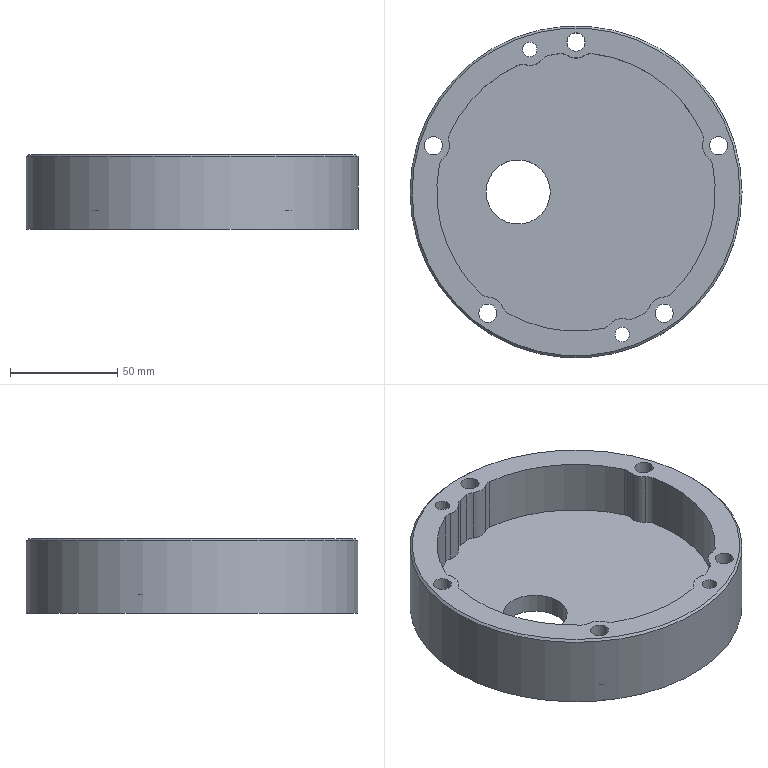Part | NX | features CBORE_HOLE 5, DATUM_CSYS 3, EXTRUDE 3, HOLE PACKAGE 2, SIMPLE HOLE 2, SKETCH 2, SYMBOLIC_THREAD 2, BLEND 1, CHAMFER 1 | 1 solid | 51 faces | box 155 x 155 x 35 mm | volume 295408 mm3 | cylinder 42 | plane 8 | cone 1 | commonest cylinder face diameters 10 x14 15 x7 130 x7 8.5 x5 14 x5 6.8 x2
STEP:
#1=CARTESIAN_POINT('',(63.725,12.809,35.));
#2=VERTEX_POINT('',#1);
#3=CARTESIAN_POINT('',(44.026,-47.82,35.));
#4=VERTEX_POINT('',#3);
#5=CARTESIAN_POINT('',(0.,0.,35.));
#6=DIRECTION('',(0.,0.,-1.));
#7=DIRECTION('',(1.,0.,0.));
#8=AXIS2_PLACEMENT_3D('',#5,#6,#7);
#9=CIRCLE('',#8,65.);
#10=EDGE_CURVE('',#2,#4,#9,.T.);
#11=ORIENTED_EDGE('',*,*,#10,.F.);
#12=CARTESIAN_POINT('',(63.725,12.809,9.));
#13=VERTEX_POINT('',#12);
#14=CARTESIAN_POINT('',(63.725,12.809,35.));
#15=DIRECTION('',(0.,0.,-1.));
#16=VECTOR('',#15,1000.);
#17=LINE('',#14,#16);
#18=EDGE_CURVE('',#2,#13,#17,.T.);
#19=ORIENTED_EDGE('',*,*,#18,.T.);
#20=CARTESIAN_POINT('',(44.026,-47.82,9.));
#21=VERTEX_POINT('',#20);
#22=CARTESIAN_POINT('',(0.,0.,9.));
#23=DIRECTION('',(0.,0.,1.));
#24=DIRECTION('',(1.,0.,0.));
#25=AXIS2_PLACEMENT_3D('',#22,#23,#24);
#26=CIRCLE('',#25,65.);
#27=EDGE_CURVE('',#21,#13,#26,.T.);
#28=ORIENTED_EDGE('',*,*,#27,.F.);
#29=CARTESIAN_POINT('',(44.026,-47.82,35.));
#30=DIRECTION('',(0.,0.,-1.));
#31=VECTOR('',#30,1000.);
#32=LINE('',#29,#31);
#33=EDGE_CURVE('',#21,#4,#32,.F.);
#34=ORIENTED_EDGE('',*,*,#33,.T.);
#35=EDGE_LOOP('',(#11,#19,#28,#34));
#36=FACE_BOUND('',#35,.T.);
#37=CARTESIAN_POINT('',(0.,0.,35.));
#38=DIRECTION('',(0.,0.,-1.));
#39=DIRECTION('',(-1.,0.,0.));
#40=AXIS2_PLACEMENT_3D('',#37,#38,#39);
#41=CYLINDRICAL_SURFACE('',#40,65.);
#42=ADVANCED_FACE('',(#36),#41,.F.);
#43=CARTESIAN_POINT('',(-31.875,-56.648,9.));
#44=VERTEX_POINT('',#43);
#45=CARTESIAN_POINT('',(12.809,-63.725,9.));
#46=VERTEX_POINT('',#45);
#47=CARTESIAN_POINT('',(0.,0.,9.));
#48=DIRECTION('',(0.,0.,1.));
#49=DIRECTION('',(1.,0.,0.));
#50=AXIS2_PLACEMENT_3D('',#47,#48,#49);
#51=CIRCLE('',#50,65.);
#52=EDGE_CURVE('',#44,#46,#51,.T.);
#53=ORIENTED_EDGE('',*,*,#52,.F.);
#54=CARTESIAN_POINT('',(-31.875,-56.648,35.));
#55=VERTEX_POINT('',#54);
#56=CARTESIAN_POINT('',(-31.875,-56.648,35.));
#57=DIRECTION('',(0.,0.,-1.));
#58=VECTOR('',#57,1000.);
#59=LINE('',#56,#58);
#60=EDGE_CURVE('',#44,#55,#59,.F.);
#61=ORIENTED_EDGE('',*,*,#60,.T.);
#62=CARTESIAN_POINT('',(12.809,-63.725,35.));
#63=VERTEX_POINT('',#62);
#64=CARTESIAN_POINT('',(0.,0.,35.));
#65=DIRECTION('',(0.,0.,-1.));
#66=DIRECTION('',(1.,0.,0.));
#67=AXIS2_PLACEMENT_3D('',#64,#65,#66);
#68=CIRCLE('',#67,65.);
#69=EDGE_CURVE('',#63,#55,#68,.T.);
#70=ORIENTED_EDGE('',*,*,#69,.F.);
#71=CARTESIAN_POINT('',(12.809,-63.725,35.));
#72=DIRECTION('',(0.,0.,-1.));
#73=VECTOR('',#72,1000.);
#74=LINE('',#71,#73);
#75=EDGE_CURVE('',#63,#46,#74,.T.);
#76=ORIENTED_EDGE('',*,*,#75,.T.);
#77=EDGE_LOOP('',(#53,#61,#70,#76));
#78=FACE_BOUND('',#77,.T.);
#79=CARTESIAN_POINT('',(0.,0.,35.));
#80=DIRECTION('',(0.,0.,-1.));
#81=DIRECTION('',(-1.,0.,0.));
#82=AXIS2_PLACEMENT_3D('',#79,#80,#81);
#83=CYLINDRICAL_SURFACE('',#82,65.);
#84=ADVANCED_FACE('',(#78),#83,.F.);
#85=CARTESIAN_POINT('',(-12.809,63.725,35.));
#86=VERTEX_POINT('',#85);
#87=CARTESIAN_POINT('',(-7.51,64.565,35.));
#88=VERTEX_POINT('',#87);
#89=CARTESIAN_POINT('',(0.,0.,35.));
#90=DIRECTION('',(0.,0.,-1.));
#91=DIRECTION('',(1.,0.,0.));
#92=AXIS2_PLACEMENT_3D('',#89,#90,#91);
#93=CIRCLE('',#92,65.);
#94=EDGE_CURVE('',#86,#88,#93,.T.);
#95=ORIENTED_EDGE('',*,*,#94,.F.);
#96=CARTESIAN_POINT('',(-12.809,63.725,9.));
#97=VERTEX_POINT('',#96);
#98=CARTESIAN_POINT('',(-12.809,63.725,35.));
#99=DIRECTION('',(0.,0.,-1.));
#100=VECTOR('',#99,1000.);
#101=LINE('',#98,#100);
#102=EDGE_CURVE('',#86,#97,#101,.T.);
#103=ORIENTED_EDGE('',*,*,#102,.T.);
#104=CARTESIAN_POINT('',(-7.51,64.565,9.));
#105=VERTEX_POINT('',#104);
#106=CARTESIAN_POINT('',(0.,0.,9.));
#107=DIRECTION('',(0.,0.,1.));
#108=DIRECTION('',(1.,0.,0.));
#109=AXIS2_PLACEMENT_3D('',#106,#107,#108);
#110=CIRCLE('',#109,65.);
#111=EDGE_CURVE('',#105,#97,#110,.T.);
#112=ORIENTED_EDGE('',*,*,#111,.F.);
#113=CARTESIAN_POINT('',(-7.51,64.565,35.));
#114=DIRECTION('',(0.,0.,-1.));
#115=VECTOR('',#114,1000.);
#116=LINE('',#113,#115);
#117=EDGE_CURVE('',#105,#88,#116,.F.);
#118=ORIENTED_EDGE('',*,*,#117,.T.);
#119=EDGE_LOOP('',(#95,#103,#112,#118));
#120=FACE_BOUND('',#119,.T.);
#121=CARTESIAN_POINT('',(0.,0.,35.));
#122=DIRECTION('',(0.,0.,-1.));
#123=DIRECTION('',(-1.,0.,0.));
#124=AXIS2_PLACEMENT_3D('',#121,#122,#123);
#125=CYLINDRICAL_SURFACE('',#124,65.);
#126=ADVANCED_FACE('',(#120),#125,.F.);
#127=CARTESIAN_POINT('',(-59.084,27.094,35.));
#128=VERTEX_POINT('',#127);
#129=CARTESIAN_POINT('',(-27.094,59.084,35.));
#130=VERTEX_POINT('',#129);
#131=CARTESIAN_POINT('',(0.,0.,35.));
#132=DIRECTION('',(0.,0.,-1.));
#133=DIRECTION('',(1.,0.,0.));
#134=AXIS2_PLACEMENT_3D('',#131,#132,#133);
#135=CIRCLE('',#134,65.);
#136=EDGE_CURVE('',#128,#130,#135,.T.);
#137=ORIENTED_EDGE('',*,*,#136,.F.);
#138=CARTESIAN_POINT('',(-59.084,27.094,9.));
#139=VERTEX_POINT('',#138);
#140=CARTESIAN_POINT('',(-59.084,27.094,35.));
#141=DIRECTION('',(0.,0.,-1.));
#142=VECTOR('',#141,1000.);
#143=LINE('',#140,#142);
#144=EDGE_CURVE('',#128,#139,#143,.T.);
#145=ORIENTED_EDGE('',*,*,#144,.T.);
#146=CARTESIAN_POINT('',(-27.094,59.084,9.));
#147=VERTEX_POINT('',#146);
#148=CARTESIAN_POINT('',(0.,0.,9.));
#149=DIRECTION('',(0.,0.,1.));
#150=DIRECTION('',(1.,0.,0.));
#151=AXIS2_PLACEMENT_3D('',#148,#149,#150);
#152=CIRCLE('',#151,65.);
#153=EDGE_CURVE('',#147,#139,#152,.T.);
#154=ORIENTED_EDGE('',*,*,#153,.F.);
#155=CARTESIAN_POINT('',(-27.094,59.084,35.));
#156=DIRECTION('',(0.,0.,-1.));
#157=VECTOR('',#156,1000.);
#158=LINE('',#155,#157);
#159=EDGE_CURVE('',#147,#130,#158,.F.);
#160=ORIENTED_EDGE('',*,*,#159,.T.);
#161=EDGE_LOOP('',(#137,#145,#154,#160));
#162=FACE_BOUND('',#161,.T.);
#163=CARTESIAN_POINT('',(0.,0.,35.));
#164=DIRECTION('',(0.,0.,-1.));
#165=DIRECTION('',(-1.,0.,0.));
#166=AXIS2_PLACEMENT_3D('',#163,#164,#165);
#167=CYLINDRICAL_SURFACE('',#166,65.);
#168=ADVANCED_FACE('',(#162),#167,.F.);
#169=CARTESIAN_POINT('',(-44.026,-47.82,35.));
#170=VERTEX_POINT('',#169);
#171=CARTESIAN_POINT('',(-63.725,12.809,35.));
#172=VERTEX_POINT('',#171);
#173=CARTESIAN_POINT('',(0.,0.,35.));
#174=DIRECTION('',(0.,0.,-1.));
#175=DIRECTION('',(1.,0.,0.));
#176=AXIS2_PLACEMENT_3D('',#173,#174,#175);
#177=CIRCLE('',#176,65.);
#178=EDGE_CURVE('',#170,#172,#177,.T.);
#179=ORIENTED_EDGE('',*,*,#178,.F.);
#180=CARTESIAN_POINT('',(-44.026,-47.82,9.));
#181=VERTEX_POINT('',#180);
#182=CARTESIAN_POINT('',(-44.026,-47.82,35.));
#183=DIRECTION('',(0.,0.,-1.));
#184=VECTOR('',#183,1000.);
#185=LINE('',#182,#184);
#186=EDGE_CURVE('',#170,#181,#185,.T.);
#187=ORIENTED_EDGE('',*,*,#186,.T.);
#188=CARTESIAN_POINT('',(-63.725,12.809,9.));
#189=VERTEX_POINT('',#188);
#190=CARTESIAN_POINT('',(0.,0.,9.));
#191=DIRECTION('',(0.,0.,1.));
#192=DIRECTION('',(1.,0.,0.));
#193=AXIS2_PLACEMENT_3D('',#190,#191,#192);
#194=CIRCLE('',#193,65.);
#195=EDGE_CURVE('',#189,#181,#194,.T.);
#196=ORIENTED_EDGE('',*,*,#195,.F.);
#197=CARTESIAN_POINT('',(-63.725,12.809,35.));
#198=DIRECTION('',(0.,0.,-1.));
#199=VECTOR('',#198,1000.);
#200=LINE('',#197,#199);
#201=EDGE_CURVE('',#189,#172,#200,.F.);
#202=ORIENTED_EDGE('',*,*,#201,.T.);
#203=EDGE_LOOP('',(#179,#187,#196,#202));
#204=FACE_BOUND('',#203,.T.);
#205=CARTESIAN_POINT('',(0.,0.,35.));
#206=DIRECTION('',(0.,0.,-1.));
#207=DIRECTION('',(-1.,0.,0.));
#208=AXIS2_PLACEMENT_3D('',#205,#206,#207);
#209=CYLINDRICAL_SURFACE('',#208,65.);
#210=ADVANCED_FACE('',(#204),#209,.F.);
#211=CARTESIAN_POINT('',(59.084,27.094,9.));
#212=VERTEX_POINT('',#211);
#213=CARTESIAN_POINT('',(7.51,64.565,9.));
#214=VERTEX_POINT('',#213);
#215=CARTESIAN_POINT('',(0.,0.,9.));
#216=DIRECTION('',(0.,0.,1.));
#217=DIRECTION('',(1.,0.,0.));
#218=AXIS2_PLACEMENT_3D('',#215,#216,#217);
#219=CIRCLE('',#218,65.);
#220=EDGE_CURVE('',#212,#214,#219,.T.);
#221=ORIENTED_EDGE('',*,*,#220,.F.);
#222=CARTESIAN_POINT('',(59.084,27.094,35.));
#223=VERTEX_POINT('',#222);
#224=CARTESIAN_POINT('',(59.084,27.094,35.));
#225=DIRECTION('',(0.,0.,-1.));
#226=VECTOR('',#225,1000.);
#227=LINE('',#224,#226);
#228=EDGE_CURVE('',#212,#223,#227,.F.);
#229=ORIENTED_EDGE('',*,*,#228,.T.);
#230=CARTESIAN_POINT('',(7.51,64.565,35.));
#231=VERTEX_POINT('',#230);
#232=CARTESIAN_POINT('',(0.,0.,35.));
#233=DIRECTION('',(0.,0.,-1.));
#234=DIRECTION('',(1.,0.,0.));
#235=AXIS2_PLACEMENT_3D('',#232,#233,#234);
#236=CIRCLE('',#235,65.);
#237=EDGE_CURVE('',#231,#223,#236,.T.);
#238=ORIENTED_EDGE('',*,*,#237,.F.);
#239=CARTESIAN_POINT('',(7.51,64.565,35.));
#240=DIRECTION('',(0.,0.,-1.));
#241=VECTOR('',#240,1000.);
#242=LINE('',#239,#241);
#243=EDGE_CURVE('',#231,#214,#242,.T.);
#244=ORIENTED_EDGE('',*,*,#243,.T.);
#245=EDGE_LOOP('',(#221,#229,#238,#244));
#246=FACE_BOUND('',#245,.T.);
#247=CARTESIAN_POINT('',(0.,0.,35.));
#248=DIRECTION('',(0.,0.,-1.));
#249=DIRECTION('',(-1.,0.,0.));
#250=AXIS2_PLACEMENT_3D('',#247,#248,#249);
#251=CYLINDRICAL_SURFACE('',#250,65.);
#252=ADVANCED_FACE('',(#246),#251,.F.);
#253=CARTESIAN_POINT('',(-12.,0.,9.));
#254=VERTEX_POINT('',#253);
#255=CARTESIAN_POINT('',(-27.,0.,9.));
#256=DIRECTION('',(0.,0.,1.));
#257=DIRECTION('',(1.,0.,0.));
#258=AXIS2_PLACEMENT_3D('',#255,#256,#257);
#259=CIRCLE('',#258,15.);
#260=EDGE_CURVE('',#254,#254,#259,.T.);
#261=ORIENTED_EDGE('',*,*,#260,.T.);
#262=EDGE_LOOP('',(#261));
#263=FACE_BOUND('',#262,.T.);
#264=CARTESIAN_POINT('',(-12.,0.,0.));
#265=VERTEX_POINT('',#264);
#266=CARTESIAN_POINT('',(-27.,0.,0.));
#267=DIRECTION('',(0.,0.,1.));
#268=DIRECTION('',(1.,0.,0.));
#269=AXIS2_PLACEMENT_3D('',#266,#267,#268);
#270=CIRCLE('',#269,15.);
#271=EDGE_CURVE('',#265,#265,#270,.T.);
#272=ORIENTED_EDGE('',*,*,#271,.F.);
#273=EDGE_LOOP('',(#272));
#274=FACE_BOUND('',#273,.T.);
#275=CARTESIAN_POINT('',(-27.,0.,9.));
#276=DIRECTION('',(0.,0.,-1.));
#277=DIRECTION('',(-1.,0.,0.));
#278=AXIS2_PLACEMENT_3D('',#275,#276,#277);
#279=CYLINDRICAL_SURFACE('',#278,15.);
#280=ADVANCED_FACE('',(#263,#274),#279,.F.);
#281=CARTESIAN_POINT('',(-34.112,-54.027,9.));
#282=VERTEX_POINT('',#281);
#283=CARTESIAN_POINT('',(-40.841,-49.137,9.));
#284=VERTEX_POINT('',#283);
#285=CARTESIAN_POINT('',(-41.145,-56.631,9.));
#286=DIRECTION('',(0.,0.,1.));
#287=DIRECTION('',(1.,0.,0.));
#288=AXIS2_PLACEMENT_3D('',#285,#286,#287);
#289=CIRCLE('',#288,7.5);
#290=EDGE_CURVE('',#282,#284,#289,.T.);
#291=ORIENTED_EDGE('',*,*,#290,.F.);
#292=CARTESIAN_POINT('',(-29.423,-52.291,9.));
#293=DIRECTION('',(0.,0.,1.));
#294=DIRECTION('',(1.,0.,0.));
#295=AXIS2_PLACEMENT_3D('',#292,#293,#294);
#296=CIRCLE('',#295,5.);
#297=EDGE_CURVE('',#282,#44,#296,.T.);
#298=ORIENTED_EDGE('',*,*,#297,.T.);
#299=ORIENTED_EDGE('',*,*,#52,.T.);
#300=CARTESIAN_POINT('',(15.747,-61.924,9.));
#301=VERTEX_POINT('',#300);
#302=CARTESIAN_POINT('',(11.824,-58.823,9.));
#303=DIRECTION('',(0.,0.,1.));
#304=DIRECTION('',(1.,0.,0.));
#305=AXIS2_PLACEMENT_3D('',#302,#303,#304);
#306=CIRCLE('',#305,5.);
#307=EDGE_CURVE('',#46,#301,#306,.T.);
#308=ORIENTED_EDGE('',*,*,#307,.T.);
#309=CARTESIAN_POINT('',(23.658,-59.353,9.));
#310=VERTEX_POINT('',#309);
#311=CARTESIAN_POINT('',(21.631,-66.574,9.));
#312=DIRECTION('',(0.,0.,1.));
#313=DIRECTION('',(1.,0.,0.));
#314=AXIS2_PLACEMENT_3D('',#311,#312,#313);
#315=CIRCLE('',#314,7.5);
#316=EDGE_CURVE('',#310,#301,#315,.T.);
#317=ORIENTED_EDGE('',*,*,#316,.F.);
#318=CARTESIAN_POINT('',(27.094,-59.084,9.));
#319=VERTEX_POINT('',#318);
#320=CARTESIAN_POINT('',(25.01,-54.539,9.));
#321=DIRECTION('',(0.,0.,1.));
#322=DIRECTION('',(1.,0.,0.));
#323=AXIS2_PLACEMENT_3D('',#320,#321,#322);
#324=CIRCLE('',#323,5.);
#325=EDGE_CURVE('',#310,#319,#324,.T.);
#326=ORIENTED_EDGE('',*,*,#325,.T.);
#327=CARTESIAN_POINT('',(31.875,-56.648,9.));
#328=VERTEX_POINT('',#327);
#329=CARTESIAN_POINT('',(0.,0.,9.));
#330=DIRECTION('',(0.,0.,1.));
#331=DIRECTION('',(1.,0.,0.));
#332=AXIS2_PLACEMENT_3D('',#329,#330,#331);
#333=CIRCLE('',#332,65.);
#334=EDGE_CURVE('',#319,#328,#333,.T.);
#335=ORIENTED_EDGE('',*,*,#334,.T.);
#336=CARTESIAN_POINT('',(34.112,-54.027,9.));
#337=VERTEX_POINT('',#336);
#338=CARTESIAN_POINT('',(29.423,-52.291,9.));
#339=DIRECTION('',(0.,0.,1.));
#340=DIRECTION('',(1.,0.,0.));
#341=AXIS2_PLACEMENT_3D('',#338,#339,#340);
#342=CIRCLE('',#341,5.);
#343=EDGE_CURVE('',#328,#337,#342,.T.);
#344=ORIENTED_EDGE('',*,*,#343,.T.);
#345=CARTESIAN_POINT('',(40.841,-49.137,9.));
#346=VERTEX_POINT('',#345);
#347=CARTESIAN_POINT('',(41.145,-56.631,9.));
#348=DIRECTION('',(0.,0.,1.));
#349=DIRECTION('',(1.,0.,0.));
#350=AXIS2_PLACEMENT_3D('',#347,#348,#349);
#351=CIRCLE('',#350,7.5);
#352=EDGE_CURVE('',#346,#337,#351,.T.);
#353=ORIENTED_EDGE('',*,*,#352,.F.);
#354=CARTESIAN_POINT('',(40.639,-44.141,9.));
#355=DIRECTION('',(0.,0.,1.));
#356=DIRECTION('',(1.,0.,0.));
#357=AXIS2_PLACEMENT_3D('',#354,#355,#356);
#358=CIRCLE('',#357,5.);
#359=EDGE_CURVE('',#346,#21,#358,.T.);
#360=ORIENTED_EDGE('',*,*,#359,.T.);
#361=ORIENTED_EDGE('',*,*,#27,.T.);
#362=CARTESIAN_POINT('',(61.924,15.747,9.));
#363=VERTEX_POINT('',#362);
#364=CARTESIAN_POINT('',(58.823,11.824,9.));
#365=DIRECTION('',(0.,0.,1.));
#366=DIRECTION('',(1.,0.,0.));
#367=AXIS2_PLACEMENT_3D('',#364,#365,#366);
#368=CIRCLE('',#367,5.);
#369=EDGE_CURVE('',#13,#363,#368,.T.);
#370=ORIENTED_EDGE('',*,*,#369,.T.);
#371=CARTESIAN_POINT('',(59.353,23.658,9.));
#372=VERTEX_POINT('',#371);
#373=CARTESIAN_POINT('',(66.574,21.631,9.));
#374=DIRECTION('',(0.,0.,1.));
#375=DIRECTION('',(1.,0.,0.));
#376=AXIS2_PLACEMENT_3D('',#373,#374,#375);
#377=CIRCLE('',#376,7.5);
#378=EDGE_CURVE('',#372,#363,#377,.T.);
#379=ORIENTED_EDGE('',*,*,#378,.F.);
#380=CARTESIAN_POINT('',(54.539,25.01,9.));
#381=DIRECTION('',(0.,0.,1.));
#382=DIRECTION('',(1.,0.,0.));
#383=AXIS2_PLACEMENT_3D('',#380,#381,#382);
#384=CIRCLE('',#383,5.);
#385=EDGE_CURVE('',#372,#212,#384,.T.);
#386=ORIENTED_EDGE('',*,*,#385,.T.);
#387=ORIENTED_EDGE('',*,*,#220,.T.);
#388=CARTESIAN_POINT('',(4.159,63.759,9.));
#389=VERTEX_POINT('',#388);
#390=CARTESIAN_POINT('',(6.932,59.598,9.));
#391=DIRECTION('',(0.,0.,1.));
#392=DIRECTION('',(1.,0.,0.));
#393=AXIS2_PLACEMENT_3D('',#390,#391,#392);
#394=CIRCLE('',#393,5.);
#395=EDGE_CURVE('',#214,#389,#394,.T.);
#396=ORIENTED_EDGE('',*,*,#395,.T.);
#397=CARTESIAN_POINT('',(-4.159,63.759,9.));
#398=VERTEX_POINT('',#397);
#399=CARTESIAN_POINT('',(0.,70.,9.));
#400=DIRECTION('',(0.,0.,1.));
#401=DIRECTION('',(1.,0.,0.));
#402=AXIS2_PLACEMENT_3D('',#399,#400,#401);
#403=CIRCLE('',#402,7.5);
#404=EDGE_CURVE('',#398,#389,#403,.T.);
#405=ORIENTED_EDGE('',*,*,#404,.F.);
#406=CARTESIAN_POINT('',(-6.932,59.598,9.));
#407=DIRECTION('',(0.,0.,1.));
#408=DIRECTION('',(1.,0.,0.));
#409=AXIS2_PLACEMENT_3D('',#406,#407,#408);
#410=CIRCLE('',#409,5.);
#411=EDGE_CURVE('',#398,#105,#410,.T.);
#412=ORIENTED_EDGE('',*,*,#411,.T.);
#413=ORIENTED_EDGE('',*,*,#111,.T.);
#414=CARTESIAN_POINT('',(-15.747,61.924,9.));
#415=VERTEX_POINT('',#414);
#416=CARTESIAN_POINT('',(-11.824,58.823,9.));
#417=DIRECTION('',(0.,0.,1.));
#418=DIRECTION('',(1.,0.,0.));
#419=AXIS2_PLACEMENT_3D('',#416,#417,#418);
#420=CIRCLE('',#419,5.);
#421=EDGE_CURVE('',#97,#415,#420,.T.);
#422=ORIENTED_EDGE('',*,*,#421,.T.);
#423=CARTESIAN_POINT('',(-23.658,59.353,9.));
#424=VERTEX_POINT('',#423);
#425=CARTESIAN_POINT('',(-21.631,66.574,9.));
#426=DIRECTION('',(0.,0.,1.));
#427=DIRECTION('',(1.,0.,0.));
#428=AXIS2_PLACEMENT_3D('',#425,#426,#427);
#429=CIRCLE('',#428,7.5);
#430=EDGE_CURVE('',#424,#415,#429,.T.);
#431=ORIENTED_EDGE('',*,*,#430,.F.);
#432=CARTESIAN_POINT('',(-25.01,54.539,9.));
#433=DIRECTION('',(0.,0.,1.));
#434=DIRECTION('',(1.,0.,0.));
#435=AXIS2_PLACEMENT_3D('',#432,#433,#434);
#436=CIRCLE('',#435,5.);
#437=EDGE_CURVE('',#424,#147,#436,.T.);
#438=ORIENTED_EDGE('',*,*,#437,.T.);
#439=ORIENTED_EDGE('',*,*,#153,.T.);
#440=CARTESIAN_POINT('',(-59.353,23.658,9.));
#441=VERTEX_POINT('',#440);
#442=CARTESIAN_POINT('',(-54.539,25.01,9.));
#443=DIRECTION('',(0.,0.,1.));
#444=DIRECTION('',(1.,0.,0.));
#445=AXIS2_PLACEMENT_3D('',#442,#443,#444);
#446=CIRCLE('',#445,5.);
#447=EDGE_CURVE('',#139,#441,#446,.T.);
#448=ORIENTED_EDGE('',*,*,#447,.T.);
#449=CARTESIAN_POINT('',(-61.924,15.747,9.));
#450=VERTEX_POINT('',#449);
#451=CARTESIAN_POINT('',(-66.574,21.631,9.));
#452=DIRECTION('',(0.,0.,1.));
#453=DIRECTION('',(1.,0.,0.));
#454=AXIS2_PLACEMENT_3D('',#451,#452,#453);
#455=CIRCLE('',#454,7.5);
#456=EDGE_CURVE('',#450,#441,#455,.T.);
#457=ORIENTED_EDGE('',*,*,#456,.F.);
#458=CARTESIAN_POINT('',(-58.823,11.824,9.));
#459=DIRECTION('',(0.,0.,1.));
#460=DIRECTION('',(1.,0.,0.));
#461=AXIS2_PLACEMENT_3D('',#458,#459,#460);
#462=CIRCLE('',#461,5.);
#463=EDGE_CURVE('',#450,#189,#462,.T.);
#464=ORIENTED_EDGE('',*,*,#463,.T.);
#465=ORIENTED_EDGE('',*,*,#195,.T.);
#466=CARTESIAN_POINT('',(-40.639,-44.141,9.));
#467=DIRECTION('',(0.,0.,1.));
#468=DIRECTION('',(1.,0.,0.));
#469=AXIS2_PLACEMENT_3D('',#466,#467,#468);
#470=CIRCLE('',#469,5.);
#471=EDGE_CURVE('',#181,#284,#470,.T.);
#472=ORIENTED_EDGE('',*,*,#471,.T.);
#473=EDGE_LOOP('',(#291,#298,#299,#308,#317,#326,#335,#344,#353,#360,#361,#370,#379,#386,#387,#396,#405,#412,#413,#422,#431,#438,#439,#448,#457,#464,#465,#472));
#474=FACE_BOUND('',#473,.T.);
#475=ORIENTED_EDGE('',*,*,#260,.F.);
#476=EDGE_LOOP('',(#475));
#477=FACE_BOUND('',#476,.T.);
#478=CARTESIAN_POINT('',(-13.5,0.,9.));
#479=DIRECTION('',(0.,0.,1.));
#480=DIRECTION('',(1.,0.,0.));
#481=AXIS2_PLACEMENT_3D('',#478,#479,#480);
#482=PLANE('',#481);
#483=ADVANCED_FACE('',(#474,#477),#482,.T.);
#484=CARTESIAN_POINT('',(25.031,-66.574,0.));
#485=VERTEX_POINT('',#484);
#486=CARTESIAN_POINT('',(21.631,-66.574,0.));
#487=DIRECTION('',(0.,0.,1.));
#488=DIRECTION('',(1.,0.,0.));
#489=AXIS2_PLACEMENT_3D('',#486,#487,#488);
#490=CIRCLE('',#489,3.4);
#491=EDGE_CURVE('',#485,#485,#490,.T.);
#492=ORIENTED_EDGE('',*,*,#491,.T.);
#493=EDGE_LOOP('',(#492));
#494=FACE_BOUND('',#493,.T.);
#495=CARTESIAN_POINT('',(-18.231,66.574,0.));
#496=VERTEX_POINT('',#495);
#497=CARTESIAN_POINT('',(-21.631,66.574,0.));
#498=DIRECTION('',(0.,0.,1.));
#499=DIRECTION('',(1.,0.,0.));
#500=AXIS2_PLACEMENT_3D('',#497,#498,#499);
#501=CIRCLE('',#500,3.4);
#502=EDGE_CURVE('',#496,#496,#501,.T.);
#503=ORIENTED_EDGE('',*,*,#502,.T.);
#504=EDGE_LOOP('',(#503));
#505=FACE_BOUND('',#504,.T.);
#506=CARTESIAN_POINT('',(73.574,21.631,0.));
#507=VERTEX_POINT('',#506);
#508=CARTESIAN_POINT('',(66.574,21.631,0.));
#509=DIRECTION('',(0.,0.,1.));
#510=DIRECTION('',(1.,0.,0.));
#511=AXIS2_PLACEMENT_3D('',#508,#509,#510);
#512=CIRCLE('',#511,7.);
#513=EDGE_CURVE('',#507,#507,#512,.T.);
#514=ORIENTED_EDGE('',*,*,#513,.T.);
#515=EDGE_LOOP('',(#514));
#516=FACE_BOUND('',#515,.T.);
#517=CARTESIAN_POINT('',(48.145,-56.631,0.));
#518=VERTEX_POINT('',#517);
#519=CARTESIAN_POINT('',(41.145,-56.631,0.));
#520=DIRECTION('',(0.,0.,1.));
#521=DIRECTION('',(1.,0.,0.));
#522=AXIS2_PLACEMENT_3D('',#519,#520,#521);
#523=CIRCLE('',#522,7.);
#524=EDGE_CURVE('',#518,#518,#523,.T.);
#525=ORIENTED_EDGE('',*,*,#524,.T.);
#526=EDGE_LOOP('',(#525));
#527=FACE_BOUND('',#526,.T.);
#528=CARTESIAN_POINT('',(-34.145,-56.631,0.));
#529=VERTEX_POINT('',#528);
#530=CARTESIAN_POINT('',(-41.145,-56.631,0.));
#531=DIRECTION('',(0.,0.,1.));
#532=DIRECTION('',(1.,0.,0.));
#533=AXIS2_PLACEMENT_3D('',#530,#531,#532);
#534=CIRCLE('',#533,7.);
#535=EDGE_CURVE('',#529,#529,#534,.T.);
#536=ORIENTED_EDGE('',*,*,#535,.T.);
#537=EDGE_LOOP('',(#536));
#538=FACE_BOUND('',#537,.T.);
#539=CARTESIAN_POINT('',(-59.574,21.631,0.));
#540=VERTEX_POINT('',#539);
#541=CARTESIAN_POINT('',(-66.574,21.631,0.));
#542=DIRECTION('',(0.,0.,1.));
#543=DIRECTION('',(1.,0.,0.));
#544=AXIS2_PLACEMENT_3D('',#541,#542,#543);
#545=CIRCLE('',#544,7.);
#546=EDGE_CURVE('',#540,#540,#545,.T.);
#547=ORIENTED_EDGE('',*,*,#546,.T.);
#548=EDGE_LOOP('',(#547));
#549=FACE_BOUND('',#548,.T.);
#550=CARTESIAN_POINT('',(7.,70.,0.));
#551=VERTEX_POINT('',#550);
#552=CARTESIAN_POINT('',(0.,70.,0.));
#553=DIRECTION('',(0.,0.,1.));
#554=DIRECTION('',(1.,0.,0.));
#555=AXIS2_PLACEMENT_3D('',#552,#553,#554);
#556=CIRCLE('',#555,7.);
#557=EDGE_CURVE('',#551,#551,#556,.T.);
#558=ORIENTED_EDGE('',*,*,#557,.T.);
#559=EDGE_LOOP('',(#558));
#560=FACE_BOUND('',#559,.T.);
#561=ORIENTED_EDGE('',*,*,#271,.T.);
#562=EDGE_LOOP('',(#561));
#563=FACE_BOUND('',#562,.T.);
#564=CARTESIAN_POINT('',(77.5,0.,0.));
#565=VERTEX_POINT('',#564);
#566=CARTESIAN_POINT('',(0.,0.,0.));
#567=DIRECTION('',(0.,0.,1.));
#568=DIRECTION('',(1.,0.,0.));
#569=AXIS2_PLACEMENT_3D('',#566,#567,#568);
#570=CIRCLE('',#569,77.5);
#571=EDGE_CURVE('',#565,#565,#570,.T.);
#572=ORIENTED_EDGE('',*,*,#571,.F.);
#573=EDGE_LOOP('',(#572));
#574=FACE_BOUND('',#573,.T.);
#575=CARTESIAN_POINT('',(-13.5,0.,0.));
#576=DIRECTION('',(0.,0.,1.));
#577=DIRECTION('',(1.,0.,0.));
#578=AXIS2_PLACEMENT_3D('',#575,#576,#577);
#579=PLANE('',#578);
#580=ADVANCED_FACE('',(#494,#505,#516,#527,#538,#549,#560,#563,#574),#579,.F.);
#581=CARTESIAN_POINT('',(77.5,0.,34.));
#582=VERTEX_POINT('',#581);
#583=CARTESIAN_POINT('',(0.,0.,34.));
#584=DIRECTION('',(0.,0.,1.));
#585=DIRECTION('',(1.,0.,0.));
#586=AXIS2_PLACEMENT_3D('',#583,#584,#585);
#587=CIRCLE('',#586,77.5);
#588=EDGE_CURVE('',#582,#582,#587,.F.);
#589=ORIENTED_EDGE('',*,*,#588,.T.);
#590=EDGE_LOOP('',(#589));
#591=FACE_BOUND('',#590,.T.);
#592=ORIENTED_EDGE('',*,*,#571,.T.);
#593=EDGE_LOOP('',(#592));
#594=FACE_BOUND('',#593,.T.);
#595=CARTESIAN_POINT('',(0.,0.,35.));
#596=DIRECTION('',(0.,0.,-1.));
#597=DIRECTION('',(-1.,0.,0.));
#598=AXIS2_PLACEMENT_3D('',#595,#596,#597);
#599=CYLINDRICAL_SURFACE('',#598,77.5);
#600=ADVANCED_FACE('',(#591,#594),#599,.T.);
#601=CARTESIAN_POINT('',(31.875,-56.648,35.));
#602=VERTEX_POINT('',#601);
#603=CARTESIAN_POINT('',(27.094,-59.084,35.));
#604=VERTEX_POINT('',#603);
#605=CARTESIAN_POINT('',(0.,0.,35.));
#606=DIRECTION('',(0.,0.,-1.));
#607=DIRECTION('',(1.,0.,0.));
#608=AXIS2_PLACEMENT_3D('',#605,#606,#607);
#609=CIRCLE('',#608,65.);
#610=EDGE_CURVE('',#602,#604,#609,.T.);
#611=ORIENTED_EDGE('',*,*,#610,.F.);
#612=CARTESIAN_POINT('',(31.875,-56.648,35.));
#613=DIRECTION('',(0.,0.,-1.));
#614=VECTOR('',#613,1000.);
#615=LINE('',#612,#614);
#616=EDGE_CURVE('',#602,#328,#615,.T.);
#617=ORIENTED_EDGE('',*,*,#616,.T.);
#618=ORIENTED_EDGE('',*,*,#334,.F.);
#619=CARTESIAN_POINT('',(27.094,-59.084,35.));
#620=DIRECTION('',(0.,0.,-1.));
#621=VECTOR('',#620,1000.);
#622=LINE('',#619,#621);
#623=EDGE_CURVE('',#319,#604,#622,.F.);
#624=ORIENTED_EDGE('',*,*,#623,.T.);
#625=EDGE_LOOP('',(#611,#617,#618,#624));
#626=FACE_BOUND('',#625,.T.);
#627=CARTESIAN_POINT('',(0.,0.,35.));
#628=DIRECTION('',(0.,0.,-1.));
#629=DIRECTION('',(-1.,0.,0.));
#630=AXIS2_PLACEMENT_3D('',#627,#628,#629);
#631=CYLINDRICAL_SURFACE('',#630,65.);
#632=ADVANCED_FACE('',(#626),#631,.F.);
#633=CARTESIAN_POINT('',(76.5,0.,35.));
#634=VERTEX_POINT('',#633);
#635=CARTESIAN_POINT('',(0.,0.,35.));
#636=DIRECTION('',(0.,0.,1.));
#637=DIRECTION('',(1.,0.,0.));
#638=AXIS2_PLACEMENT_3D('',#635,#636,#637);
#639=CIRCLE('',#638,76.5);
#640=EDGE_CURVE('',#634,#634,#639,.T.);
#641=ORIENTED_EDGE('',*,*,#640,.T.);
#642=EDGE_LOOP('',(#641));
#643=FACE_BOUND('',#642,.T.);
#644=CARTESIAN_POINT('',(25.031,-66.574,35.));
#645=VERTEX_POINT('',#644);
#646=CARTESIAN_POINT('',(21.631,-66.574,35.));
#647=DIRECTION('',(0.,0.,1.));
#648=DIRECTION('',(1.,0.,0.));
#649=AXIS2_PLACEMENT_3D('',#646,#647,#648);
#650=CIRCLE('',#649,3.4);
#651=EDGE_CURVE('',#645,#645,#650,.T.);
#652=ORIENTED_EDGE('',*,*,#651,.F.);
#653=EDGE_LOOP('',(#652));
#654=FACE_BOUND('',#653,.T.);
#655=CARTESIAN_POINT('',(-18.231,66.574,35.));
#656=VERTEX_POINT('',#655);
#657=CARTESIAN_POINT('',(-21.631,66.574,35.));
#658=DIRECTION('',(0.,0.,1.));
#659=DIRECTION('',(1.,0.,0.));
#660=AXIS2_PLACEMENT_3D('',#657,#658,#659);
#661=CIRCLE('',#660,3.4);
#662=EDGE_CURVE('',#656,#656,#661,.T.);
#663=ORIENTED_EDGE('',*,*,#662,.F.);
#664=EDGE_LOOP('',(#663));
#665=FACE_BOUND('',#664,.T.);
#666=CARTESIAN_POINT('',(70.824,21.631,35.));
#667=VERTEX_POINT('',#666);
#668=CARTESIAN_POINT('',(66.574,21.631,35.));
#669=DIRECTION('',(0.,0.,1.));
#670=DIRECTION('',(1.,0.,0.));
#671=AXIS2_PLACEMENT_3D('',#668,#669,#670);
#672=CIRCLE('',#671,4.25);
#673=EDGE_CURVE('',#667,#667,#672,.T.);
#674=ORIENTED_EDGE('',*,*,#673,.F.);
#675=EDGE_LOOP('',(#674));
#676=FACE_BOUND('',#675,.T.);
#677=CARTESIAN_POINT('',(45.395,-56.631,35.));
#678=VERTEX_POINT('',#677);
#679=CARTESIAN_POINT('',(41.145,-56.631,35.));
#680=DIRECTION('',(0.,0.,1.));
#681=DIRECTION('',(1.,0.,0.));
#682=AXIS2_PLACEMENT_3D('',#679,#680,#681);
#683=CIRCLE('',#682,4.25);
#684=EDGE_CURVE('',#678,#678,#683,.T.);
#685=ORIENTED_EDGE('',*,*,#684,.F.);
#686=EDGE_LOOP('',(#685));
#687=FACE_BOUND('',#686,.T.);
#688=CARTESIAN_POINT('',(-36.895,-56.631,35.));
#689=VERTEX_POINT('',#688);
#690=CARTESIAN_POINT('',(-41.145,-56.631,35.));
#691=DIRECTION('',(0.,0.,1.));
#692=DIRECTION('',(1.,0.,0.));
#693=AXIS2_PLACEMENT_3D('',#690,#691,#692);
#694=CIRCLE('',#693,4.25);
#695=EDGE_CURVE('',#689,#689,#694,.T.);
#696=ORIENTED_EDGE('',*,*,#695,.F.);
#697=EDGE_LOOP('',(#696));
#698=FACE_BOUND('',#697,.T.);
#699=CARTESIAN_POINT('',(-62.324,21.631,35.));
#700=VERTEX_POINT('',#699);
#701=CARTESIAN_POINT('',(-66.574,21.631,35.));
#702=DIRECTION('',(0.,0.,1.));
#703=DIRECTION('',(1.,0.,0.));
#704=AXIS2_PLACEMENT_3D('',#701,#702,#703);
#705=CIRCLE('',#704,4.25);
#706=EDGE_CURVE('',#700,#700,#705,.T.);
#707=ORIENTED_EDGE('',*,*,#706,.F.);
#708=EDGE_LOOP('',(#707));
#709=FACE_BOUND('',#708,.T.);
#710=CARTESIAN_POINT('',(4.25,70.,35.));
#711=VERTEX_POINT('',#710);
#712=CARTESIAN_POINT('',(0.,70.,35.));
#713=DIRECTION('',(0.,0.,1.));
#714=DIRECTION('',(1.,0.,0.));
#715=AXIS2_PLACEMENT_3D('',#712,#713,#714);
#716=CIRCLE('',#715,4.25);
#717=EDGE_CURVE('',#711,#711,#716,.T.);
#718=ORIENTED_EDGE('',*,*,#717,.F.);
#719=EDGE_LOOP('',(#718));
#720=FACE_BOUND('',#719,.T.);
#721=CARTESIAN_POINT('',(4.159,63.759,35.));
#722=VERTEX_POINT('',#721);
#723=CARTESIAN_POINT('',(-4.159,63.759,35.));
#724=VERTEX_POINT('',#723);
#725=CARTESIAN_POINT('',(0.,70.,35.));
#726=DIRECTION('',(0.,0.,-1.));
#727=DIRECTION('',(1.,0.,0.));
#728=AXIS2_PLACEMENT_3D('',#725,#726,#727);
#729=CIRCLE('',#728,7.5);
#730=EDGE_CURVE('',#722,#724,#729,.T.);
#731=ORIENTED_EDGE('',*,*,#730,.F.);
#732=CARTESIAN_POINT('',(6.932,59.598,35.));
#733=DIRECTION('',(0.,0.,1.));
#734=DIRECTION('',(1.,0.,0.));
#735=AXIS2_PLACEMENT_3D('',#732,#733,#734);
#736=CIRCLE('',#735,5.);
#737=EDGE_CURVE('',#722,#231,#736,.F.);
#738=ORIENTED_EDGE('',*,*,#737,.T.);
#739=ORIENTED_EDGE('',*,*,#237,.T.);
#740=CARTESIAN_POINT('',(59.353,23.658,35.));
#741=VERTEX_POINT('',#740);
#742=CARTESIAN_POINT('',(54.539,25.01,35.));
#743=DIRECTION('',(0.,0.,1.));
#744=DIRECTION('',(1.,0.,0.));
#745=AXIS2_PLACEMENT_3D('',#742,#743,#744);
#746=CIRCLE('',#745,5.);
#747=EDGE_CURVE('',#223,#741,#746,.F.);
#748=ORIENTED_EDGE('',*,*,#747,.T.);
#749=CARTESIAN_POINT('',(61.924,15.747,35.));
#750=VERTEX_POINT('',#749);
#751=CARTESIAN_POINT('',(66.574,21.631,35.));
#752=DIRECTION('',(0.,0.,-1.));
#753=DIRECTION('',(1.,0.,0.));
#754=AXIS2_PLACEMENT_3D('',#751,#752,#753);
#755=CIRCLE('',#754,7.5);
#756=EDGE_CURVE('',#750,#741,#755,.T.);
#757=ORIENTED_EDGE('',*,*,#756,.F.);
#758=CARTESIAN_POINT('',(58.823,11.824,35.));
#759=DIRECTION('',(0.,0.,1.));
#760=DIRECTION('',(1.,0.,0.));
#761=AXIS2_PLACEMENT_3D('',#758,#759,#760);
#762=CIRCLE('',#761,5.);
#763=EDGE_CURVE('',#750,#2,#762,.F.);
#764=ORIENTED_EDGE('',*,*,#763,.T.);
#765=ORIENTED_EDGE('',*,*,#10,.T.);
#766=CARTESIAN_POINT('',(40.841,-49.137,35.));
#767=VERTEX_POINT('',#766);
#768=CARTESIAN_POINT('',(40.639,-44.141,35.));
#769=DIRECTION('',(0.,0.,1.));
#770=DIRECTION('',(1.,0.,0.));
#771=AXIS2_PLACEMENT_3D('',#768,#769,#770);
#772=CIRCLE('',#771,5.);
#773=EDGE_CURVE('',#4,#767,#772,.F.);
#774=ORIENTED_EDGE('',*,*,#773,.T.);
#775=CARTESIAN_POINT('',(34.112,-54.027,35.));
#776=VERTEX_POINT('',#775);
#777=CARTESIAN_POINT('',(41.145,-56.631,35.));
#778=DIRECTION('',(0.,0.,-1.));
#779=DIRECTION('',(1.,0.,0.));
#780=AXIS2_PLACEMENT_3D('',#777,#778,#779);
#781=CIRCLE('',#780,7.5);
#782=EDGE_CURVE('',#776,#767,#781,.T.);
#783=ORIENTED_EDGE('',*,*,#782,.F.);
#784=CARTESIAN_POINT('',(29.423,-52.291,35.));
#785=DIRECTION('',(0.,0.,1.));
#786=DIRECTION('',(1.,0.,0.));
#787=AXIS2_PLACEMENT_3D('',#784,#785,#786);
#788=CIRCLE('',#787,5.);
#789=EDGE_CURVE('',#776,#602,#788,.F.);
#790=ORIENTED_EDGE('',*,*,#789,.T.);
#791=ORIENTED_EDGE('',*,*,#610,.T.);
#792=CARTESIAN_POINT('',(23.658,-59.353,35.));
#793=VERTEX_POINT('',#792);
#794=CARTESIAN_POINT('',(25.01,-54.539,35.));
#795=DIRECTION('',(0.,0.,1.));
#796=DIRECTION('',(1.,0.,0.));
#797=AXIS2_PLACEMENT_3D('',#794,#795,#796);
#798=CIRCLE('',#797,5.);
#799=EDGE_CURVE('',#604,#793,#798,.F.);
#800=ORIENTED_EDGE('',*,*,#799,.T.);
#801=CARTESIAN_POINT('',(15.747,-61.924,35.));
#802=VERTEX_POINT('',#801);
#803=CARTESIAN_POINT('',(21.631,-66.574,35.));
#804=DIRECTION('',(0.,0.,-1.));
#805=DIRECTION('',(1.,0.,0.));
#806=AXIS2_PLACEMENT_3D('',#803,#804,#805);
#807=CIRCLE('',#806,7.5);
#808=EDGE_CURVE('',#802,#793,#807,.T.);
#809=ORIENTED_EDGE('',*,*,#808,.F.);
#810=CARTESIAN_POINT('',(11.824,-58.823,35.));
#811=DIRECTION('',(0.,0.,1.));
#812=DIRECTION('',(1.,0.,0.));
#813=AXIS2_PLACEMENT_3D('',#810,#811,#812);
#814=CIRCLE('',#813,5.);
#815=EDGE_CURVE('',#802,#63,#814,.F.);
#816=ORIENTED_EDGE('',*,*,#815,.T.);
#817=ORIENTED_EDGE('',*,*,#69,.T.);
#818=CARTESIAN_POINT('',(-34.112,-54.027,35.));
#819=VERTEX_POINT('',#818);
#820=CARTESIAN_POINT('',(-29.423,-52.291,35.));
#821=DIRECTION('',(0.,0.,1.));
#822=DIRECTION('',(1.,0.,0.));
#823=AXIS2_PLACEMENT_3D('',#820,#821,#822);
#824=CIRCLE('',#823,5.);
#825=EDGE_CURVE('',#55,#819,#824,.F.);
#826=ORIENTED_EDGE('',*,*,#825,.T.);
#827=CARTESIAN_POINT('',(-40.841,-49.137,35.));
#828=VERTEX_POINT('',#827);
#829=CARTESIAN_POINT('',(-41.145,-56.631,35.));
#830=DIRECTION('',(0.,0.,-1.));
#831=DIRECTION('',(1.,0.,0.));
#832=AXIS2_PLACEMENT_3D('',#829,#830,#831);
#833=CIRCLE('',#832,7.5);
#834=EDGE_CURVE('',#828,#819,#833,.T.);
#835=ORIENTED_EDGE('',*,*,#834,.F.);
#836=CARTESIAN_POINT('',(-40.639,-44.141,35.));
#837=DIRECTION('',(0.,0.,1.));
#838=DIRECTION('',(1.,0.,0.));
#839=AXIS2_PLACEMENT_3D('',#836,#837,#838);
#840=CIRCLE('',#839,5.);
#841=EDGE_CURVE('',#828,#170,#840,.F.);
#842=ORIENTED_EDGE('',*,*,#841,.T.);
#843=ORIENTED_EDGE('',*,*,#178,.T.);
#844=CARTESIAN_POINT('',(-61.924,15.747,35.));
#845=VERTEX_POINT('',#844);
#846=CARTESIAN_POINT('',(-58.823,11.824,35.));
#847=DIRECTION('',(0.,0.,1.));
#848=DIRECTION('',(1.,0.,0.));
#849=AXIS2_PLACEMENT_3D('',#846,#847,#848);
#850=CIRCLE('',#849,5.);
#851=EDGE_CURVE('',#172,#845,#850,.F.);
#852=ORIENTED_EDGE('',*,*,#851,.T.);
#853=CARTESIAN_POINT('',(-59.353,23.658,35.));
#854=VERTEX_POINT('',#853);
#855=CARTESIAN_POINT('',(-66.574,21.631,35.));
#856=DIRECTION('',(0.,0.,-1.));
#857=DIRECTION('',(1.,0.,0.));
#858=AXIS2_PLACEMENT_3D('',#855,#856,#857);
#859=CIRCLE('',#858,7.5);
#860=EDGE_CURVE('',#854,#845,#859,.T.);
#861=ORIENTED_EDGE('',*,*,#860,.F.);
#862=CARTESIAN_POINT('',(-54.539,25.01,35.));
#863=DIRECTION('',(0.,0.,1.));
#864=DIRECTION('',(1.,0.,0.));
#865=AXIS2_PLACEMENT_3D('',#862,#863,#864);
#866=CIRCLE('',#865,5.);
#867=EDGE_CURVE('',#854,#128,#866,.F.);
#868=ORIENTED_EDGE('',*,*,#867,.T.);
#869=ORIENTED_EDGE('',*,*,#136,.T.);
#870=CARTESIAN_POINT('',(-23.658,59.353,35.));
#871=VERTEX_POINT('',#870);
#872=CARTESIAN_POINT('',(-25.01,54.539,35.));
#873=DIRECTION('',(0.,0.,1.));
#874=DIRECTION('',(1.,0.,0.));
#875=AXIS2_PLACEMENT_3D('',#872,#873,#874);
#876=CIRCLE('',#875,5.);
#877=EDGE_CURVE('',#130,#871,#876,.F.);
#878=ORIENTED_EDGE('',*,*,#877,.T.);
#879=CARTESIAN_POINT('',(-15.747,61.924,35.));
#880=VERTEX_POINT('',#879);
#881=CARTESIAN_POINT('',(-21.631,66.574,35.));
#882=DIRECTION('',(0.,0.,-1.));
#883=DIRECTION('',(1.,0.,0.));
#884=AXIS2_PLACEMENT_3D('',#881,#882,#883);
#885=CIRCLE('',#884,7.5);
#886=EDGE_CURVE('',#880,#871,#885,.T.);
#887=ORIENTED_EDGE('',*,*,#886,.F.);
#888=CARTESIAN_POINT('',(-11.824,58.823,35.));
#889=DIRECTION('',(0.,0.,1.));
#890=DIRECTION('',(1.,0.,0.));
#891=AXIS2_PLACEMENT_3D('',#888,#889,#890);
#892=CIRCLE('',#891,5.);
#893=EDGE_CURVE('',#880,#86,#892,.F.);
#894=ORIENTED_EDGE('',*,*,#893,.T.);
#895=ORIENTED_EDGE('',*,*,#94,.T.);
#896=CARTESIAN_POINT('',(-6.932,59.598,35.));
#897=DIRECTION('',(0.,0.,1.));
#898=DIRECTION('',(1.,0.,0.));
#899=AXIS2_PLACEMENT_3D('',#896,#897,#898);
#900=CIRCLE('',#899,5.);
#901=EDGE_CURVE('',#88,#724,#900,.F.);
#902=ORIENTED_EDGE('',*,*,#901,.T.);
#903=EDGE_LOOP('',(#731,#738,#739,#748,#757,#764,#765,#774,#783,#790,#791,#800,#809,#816,#817,#826,#835,#842,#843,#852,#861,#868,#869,#878,#887,#894,#895,#902));
#904=FACE_BOUND('',#903,.T.);
#905=CARTESIAN_POINT('',(33.287,10.816,35.));
#906=DIRECTION('',(0.,0.,1.));
#907=DIRECTION('',(1.,0.,0.));
#908=AXIS2_PLACEMENT_3D('',#905,#906,#907);
#909=PLANE('',#908);
#910=ADVANCED_FACE('',(#643,#654,#665,#676,#687,#698,#709,#720,#904),#909,.T.);
#911=ORIENTED_EDGE('',*,*,#352,.T.);
#912=CARTESIAN_POINT('',(34.112,-54.027,35.));
#913=DIRECTION('',(0.,0.,-1.));
#914=VECTOR('',#913,1000.);
#915=LINE('',#912,#914);
#916=EDGE_CURVE('',#337,#776,#915,.F.);
#917=ORIENTED_EDGE('',*,*,#916,.T.);
#918=ORIENTED_EDGE('',*,*,#782,.T.);
#919=CARTESIAN_POINT('',(40.841,-49.137,35.));
#920=DIRECTION('',(0.,0.,-1.));
#921=VECTOR('',#920,1000.);
#922=LINE('',#919,#921);
#923=EDGE_CURVE('',#767,#346,#922,.T.);
#924=ORIENTED_EDGE('',*,*,#923,.T.);
#925=EDGE_LOOP('',(#911,#917,#918,#924));
#926=FACE_BOUND('',#925,.T.);
#927=CARTESIAN_POINT('',(41.145,-56.631,35.));
#928=DIRECTION('',(0.,0.,-1.));
#929=DIRECTION('',(-1.,0.,0.));
#930=AXIS2_PLACEMENT_3D('',#927,#928,#929);
#931=CYLINDRICAL_SURFACE('',#930,7.5);
#932=ADVANCED_FACE('',(#926),#931,.T.);
#933=ORIENTED_EDGE('',*,*,#404,.T.);
#934=CARTESIAN_POINT('',(4.159,63.759,35.));
#935=DIRECTION('',(0.,0.,-1.));
#936=VECTOR('',#935,1000.);
#937=LINE('',#934,#936);
#938=EDGE_CURVE('',#389,#722,#937,.F.);
#939=ORIENTED_EDGE('',*,*,#938,.T.);
#940=ORIENTED_EDGE('',*,*,#730,.T.);
#941=CARTESIAN_POINT('',(-4.159,63.759,35.));
#942=DIRECTION('',(0.,0.,-1.));
#943=VECTOR('',#942,1000.);
#944=LINE('',#941,#943);
#945=EDGE_CURVE('',#724,#398,#944,.T.);
#946=ORIENTED_EDGE('',*,*,#945,.T.);
#947=EDGE_LOOP('',(#933,#939,#940,#946));
#948=FACE_BOUND('',#947,.T.);
#949=CARTESIAN_POINT('',(0.,70.,35.));
#950=DIRECTION('',(0.,0.,-1.));
#951=DIRECTION('',(-1.,0.,0.));
#952=AXIS2_PLACEMENT_3D('',#949,#950,#951);
#953=CYLINDRICAL_SURFACE('',#952,7.5);
#954=ADVANCED_FACE('',(#948),#953,.T.);
#955=ORIENTED_EDGE('',*,*,#834,.T.);
#956=CARTESIAN_POINT('',(-34.112,-54.027,35.));
#957=DIRECTION('',(0.,0.,-1.));
#958=VECTOR('',#957,1000.);
#959=LINE('',#956,#958);
#960=EDGE_CURVE('',#819,#282,#959,.T.);
#961=ORIENTED_EDGE('',*,*,#960,.T.);
#962=ORIENTED_EDGE('',*,*,#290,.T.);
#963=CARTESIAN_POINT('',(-40.841,-49.137,35.));
#964=DIRECTION('',(0.,0.,-1.));
#965=VECTOR('',#964,1000.);
#966=LINE('',#963,#965);
#967=EDGE_CURVE('',#284,#828,#966,.F.);
#968=ORIENTED_EDGE('',*,*,#967,.T.);
#969=EDGE_LOOP('',(#955,#961,#962,#968));
#970=FACE_BOUND('',#969,.T.);
#971=CARTESIAN_POINT('',(-41.145,-56.631,35.));
#972=DIRECTION('',(0.,0.,-1.));
#973=DIRECTION('',(-1.,0.,0.));
#974=AXIS2_PLACEMENT_3D('',#971,#972,#973);
#975=CYLINDRICAL_SURFACE('',#974,7.5);
#976=ADVANCED_FACE('',(#970),#975,.T.);
#977=ORIENTED_EDGE('',*,*,#860,.T.);
#978=CARTESIAN_POINT('',(-61.924,15.747,35.));
#979=DIRECTION('',(0.,0.,-1.));
#980=VECTOR('',#979,1000.);
#981=LINE('',#978,#980);
#982=EDGE_CURVE('',#845,#450,#981,.T.);
#983=ORIENTED_EDGE('',*,*,#982,.T.);
#984=ORIENTED_EDGE('',*,*,#456,.T.);
#985=CARTESIAN_POINT('',(-59.353,23.658,35.));
#986=DIRECTION('',(0.,0.,-1.));
#987=VECTOR('',#986,1000.);
#988=LINE('',#985,#987);
#989=EDGE_CURVE('',#441,#854,#988,.F.);
#990=ORIENTED_EDGE('',*,*,#989,.T.);
#991=EDGE_LOOP('',(#977,#983,#984,#990));
#992=FACE_BOUND('',#991,.T.);
#993=CARTESIAN_POINT('',(-66.574,21.631,35.));
#994=DIRECTION('',(0.,0.,-1.));
#995=DIRECTION('',(-1.,0.,0.));
#996=AXIS2_PLACEMENT_3D('',#993,#994,#995);
#997=CYLINDRICAL_SURFACE('',#996,7.5);
#998=ADVANCED_FACE('',(#992),#997,.T.);
#999=ORIENTED_EDGE('',*,*,#430,.T.);
#1000=CARTESIAN_POINT('',(-15.747,61.924,35.));
#1001=DIRECTION('',(0.,0.,-1.));
#1002=VECTOR('',#1001,1000.);
#1003=LINE('',#1000,#1002);
#1004=EDGE_CURVE('',#415,#880,#1003,.F.);
#1005=ORIENTED_EDGE('',*,*,#1004,.T.);
#1006=ORIENTED_EDGE('',*,*,#886,.T.);
#1007=CARTESIAN_POINT('',(-23.658,59.353,35.));
#1008=DIRECTION('',(0.,0.,-1.));
#1009=VECTOR('',#1008,1000.);
#1010=LINE('',#1007,#1009);
#1011=EDGE_CURVE('',#871,#424,#1010,.T.);
#1012=ORIENTED_EDGE('',*,*,#1011,.T.);
#1013=EDGE_LOOP('',(#999,#1005,#1006,#1012));
#1014=FACE_BOUND('',#1013,.T.);
#1015=CARTESIAN_POINT('',(-21.631,66.574,35.));
#1016=DIRECTION('',(0.,0.,-1.));
#1017=DIRECTION('',(-1.,0.,0.));
#1018=AXIS2_PLACEMENT_3D('',#1015,#1016,#1017);
#1019=CYLINDRICAL_SURFACE('',#1018,7.5);
#1020=ADVANCED_FACE('',(#1014),#1019,.T.);
#1021=ORIENTED_EDGE('',*,*,#316,.T.);
#1022=CARTESIAN_POINT('',(15.747,-61.924,35.));
#1023=DIRECTION('',(0.,0.,-1.));
#1024=VECTOR('',#1023,1000.);
#1025=LINE('',#1022,#1024);
#1026=EDGE_CURVE('',#301,#802,#1025,.F.);
#1027=ORIENTED_EDGE('',*,*,#1026,.T.);
#1028=ORIENTED_EDGE('',*,*,#808,.T.);
#1029=CARTESIAN_POINT('',(23.658,-59.353,35.));
#1030=DIRECTION('',(0.,0.,-1.));
#1031=VECTOR('',#1030,1000.);
#1032=LINE('',#1029,#1031);
#1033=EDGE_CURVE('',#793,#310,#1032,.T.);
#1034=ORIENTED_EDGE('',*,*,#1033,.T.);
#1035=EDGE_LOOP('',(#1021,#1027,#1028,#1034));
#1036=FACE_BOUND('',#1035,.T.);
#1037=CARTESIAN_POINT('',(21.631,-66.574,35.));
#1038=DIRECTION('',(0.,0.,-1.));
#1039=DIRECTION('',(-1.,0.,0.));
#1040=AXIS2_PLACEMENT_3D('',#1037,#1038,#1039);
#1041=CYLINDRICAL_SURFACE('',#1040,7.5);
#1042=ADVANCED_FACE('',(#1036),#1041,.T.);
#1043=ORIENTED_EDGE('',*,*,#378,.T.);
#1044=CARTESIAN_POINT('',(61.924,15.747,35.));
#1045=DIRECTION('',(0.,0.,-1.));
#1046=VECTOR('',#1045,1000.);
#1047=LINE('',#1044,#1046);
#1048=EDGE_CURVE('',#363,#750,#1047,.F.);
#1049=ORIENTED_EDGE('',*,*,#1048,.T.);
#1050=ORIENTED_EDGE('',*,*,#756,.T.);
#1051=CARTESIAN_POINT('',(59.353,23.658,35.));
#1052=DIRECTION('',(0.,0.,-1.));
#1053=VECTOR('',#1052,1000.);
#1054=LINE('',#1051,#1053);
#1055=EDGE_CURVE('',#741,#372,#1054,.T.);
#1056=ORIENTED_EDGE('',*,*,#1055,.T.);
#1057=EDGE_LOOP('',(#1043,#1049,#1050,#1056));
#1058=FACE_BOUND('',#1057,.T.);
#1059=CARTESIAN_POINT('',(66.574,21.631,35.));
#1060=DIRECTION('',(0.,0.,-1.));
#1061=DIRECTION('',(-1.,0.,0.));
#1062=AXIS2_PLACEMENT_3D('',#1059,#1060,#1061);
#1063=CYLINDRICAL_SURFACE('',#1062,7.5);
#1064=ADVANCED_FACE('',(#1058),#1063,.T.);
#1065=ORIENTED_EDGE('',*,*,#717,.T.);
#1066=EDGE_LOOP('',(#1065));
#1067=FACE_BOUND('',#1066,.T.);
#1068=CARTESIAN_POINT('',(4.25,70.,9.));
#1069=VERTEX_POINT('',#1068);
#1070=CARTESIAN_POINT('',(0.,70.,9.));
#1071=DIRECTION('',(0.,0.,1.));
#1072=DIRECTION('',(1.,0.,0.));
#1073=AXIS2_PLACEMENT_3D('',#1070,#1071,#1072);
#1074=CIRCLE('',#1073,4.25);
#1075=EDGE_CURVE('',#1069,#1069,#1074,.F.);
#1076=ORIENTED_EDGE('',*,*,#1075,.T.);
#1077=EDGE_LOOP('',(#1076));
#1078=FACE_BOUND('',#1077,.T.);
#1079=CARTESIAN_POINT('',(0.,70.,117.528));
#1080=DIRECTION('',(0.,0.,1.));
#1081=DIRECTION('',(1.,0.,0.));
#1082=AXIS2_PLACEMENT_3D('',#1079,#1080,#1081);
#1083=CYLINDRICAL_SURFACE('',#1082,4.25);
#1084=ADVANCED_FACE('',(#1067,#1078),#1083,.F.);
#1085=ORIENTED_EDGE('',*,*,#1075,.F.);
#1086=EDGE_LOOP('',(#1085));
#1087=FACE_BOUND('',#1086,.T.);
#1088=CARTESIAN_POINT('',(7.,70.,9.));
#1089=VERTEX_POINT('',#1088);
#1090=CARTESIAN_POINT('',(0.,70.,9.));
#1091=DIRECTION('',(0.,0.,1.));
#1092=DIRECTION('',(1.,0.,0.));
#1093=AXIS2_PLACEMENT_3D('',#1090,#1091,#1092);
#1094=CIRCLE('',#1093,7.);
#1095=EDGE_CURVE('',#1089,#1089,#1094,.F.);
#1096=ORIENTED_EDGE('',*,*,#1095,.T.);
#1097=EDGE_LOOP('',(#1096));
#1098=FACE_BOUND('',#1097,.T.);
#1099=CARTESIAN_POINT('',(0.,70.,9.));
#1100=DIRECTION('',(0.,0.,1.));
#1101=DIRECTION('',(1.,0.,0.));
#1102=AXIS2_PLACEMENT_3D('',#1099,#1100,#1101);
#1103=PLANE('',#1102);
#1104=ADVANCED_FACE('',(#1087,#1098),#1103,.F.);
#1105=ORIENTED_EDGE('',*,*,#1095,.F.);
#1106=EDGE_LOOP('',(#1105));
#1107=FACE_BOUND('',#1106,.T.);
#1108=ORIENTED_EDGE('',*,*,#557,.F.);
#1109=EDGE_LOOP('',(#1108));
#1110=FACE_BOUND('',#1109,.T.);
#1111=CARTESIAN_POINT('',(0.,70.,0.));
#1112=DIRECTION('',(0.,0.,1.));
#1113=DIRECTION('',(1.,0.,0.));
#1114=AXIS2_PLACEMENT_3D('',#1111,#1112,#1113);
#1115=CYLINDRICAL_SURFACE('',#1114,7.);
#1116=ADVANCED_FACE('',(#1107,#1110),#1115,.F.);
#1117=ORIENTED_EDGE('',*,*,#706,.T.);
#1118=EDGE_LOOP('',(#1117));
#1119=FACE_BOUND('',#1118,.T.);
#1120=CARTESIAN_POINT('',(-62.324,21.631,9.));
#1121=VERTEX_POINT('',#1120);
#1122=CARTESIAN_POINT('',(-66.574,21.631,9.));
#1123=DIRECTION('',(0.,0.,1.));
#1124=DIRECTION('',(1.,0.,0.));
#1125=AXIS2_PLACEMENT_3D('',#1122,#1123,#1124);
#1126=CIRCLE('',#1125,4.25);
#1127=EDGE_CURVE('',#1121,#1121,#1126,.F.);
#1128=ORIENTED_EDGE('',*,*,#1127,.T.);
#1129=EDGE_LOOP('',(#1128));
#1130=FACE_BOUND('',#1129,.T.);
#1131=CARTESIAN_POINT('',(-66.574,21.631,117.528));
#1132=DIRECTION('',(0.,0.,1.));
#1133=DIRECTION('',(1.,0.,0.));
#1134=AXIS2_PLACEMENT_3D('',#1131,#1132,#1133);
#1135=CYLINDRICAL_SURFACE('',#1134,4.25);
#1136=ADVANCED_FACE('',(#1119,#1130),#1135,.F.);
#1137=ORIENTED_EDGE('',*,*,#1127,.F.);
#1138=EDGE_LOOP('',(#1137));
#1139=FACE_BOUND('',#1138,.T.);
#1140=CARTESIAN_POINT('',(-59.574,21.631,9.));
#1141=VERTEX_POINT('',#1140);
#1142=CARTESIAN_POINT('',(-66.574,21.631,9.));
#1143=DIRECTION('',(0.,0.,1.));
#1144=DIRECTION('',(1.,0.,0.));
#1145=AXIS2_PLACEMENT_3D('',#1142,#1143,#1144);
#1146=CIRCLE('',#1145,7.);
#1147=EDGE_CURVE('',#1141,#1141,#1146,.F.);
#1148=ORIENTED_EDGE('',*,*,#1147,.T.);
#1149=EDGE_LOOP('',(#1148));
#1150=FACE_BOUND('',#1149,.T.);
#1151=CARTESIAN_POINT('',(-66.574,21.631,9.));
#1152=DIRECTION('',(0.,0.,1.));
#1153=DIRECTION('',(1.,0.,0.));
#1154=AXIS2_PLACEMENT_3D('',#1151,#1152,#1153);
#1155=PLANE('',#1154);
#1156=ADVANCED_FACE('',(#1139,#1150),#1155,.F.);
#1157=ORIENTED_EDGE('',*,*,#1147,.F.);
#1158=EDGE_LOOP('',(#1157));
#1159=FACE_BOUND('',#1158,.T.);
#1160=ORIENTED_EDGE('',*,*,#546,.F.);
#1161=EDGE_LOOP('',(#1160));
#1162=FACE_BOUND('',#1161,.T.);
#1163=CARTESIAN_POINT('',(-66.574,21.631,0.));
#1164=DIRECTION('',(0.,0.,1.));
#1165=DIRECTION('',(1.,0.,0.));
#1166=AXIS2_PLACEMENT_3D('',#1163,#1164,#1165);
#1167=CYLINDRICAL_SURFACE('',#1166,7.);
#1168=ADVANCED_FACE('',(#1159,#1162),#1167,.F.);
#1169=ORIENTED_EDGE('',*,*,#695,.T.);
#1170=EDGE_LOOP('',(#1169));
#1171=FACE_BOUND('',#1170,.T.);
#1172=CARTESIAN_POINT('',(-36.895,-56.631,9.));
#1173=VERTEX_POINT('',#1172);
#1174=CARTESIAN_POINT('',(-41.145,-56.631,9.));
#1175=DIRECTION('',(0.,0.,1.));
#1176=DIRECTION('',(1.,0.,0.));
#1177=AXIS2_PLACEMENT_3D('',#1174,#1175,#1176);
#1178=CIRCLE('',#1177,4.25);
#1179=EDGE_CURVE('',#1173,#1173,#1178,.F.);
#1180=ORIENTED_EDGE('',*,*,#1179,.T.);
#1181=EDGE_LOOP('',(#1180));
#1182=FACE_BOUND('',#1181,.T.);
#1183=CARTESIAN_POINT('',(-41.145,-56.631,117.528));
#1184=DIRECTION('',(0.,0.,1.));
#1185=DIRECTION('',(1.,0.,0.));
#1186=AXIS2_PLACEMENT_3D('',#1183,#1184,#1185);
#1187=CYLINDRICAL_SURFACE('',#1186,4.25);
#1188=ADVANCED_FACE('',(#1171,#1182),#1187,.F.);
#1189=ORIENTED_EDGE('',*,*,#1179,.F.);
#1190=EDGE_LOOP('',(#1189));
#1191=FACE_BOUND('',#1190,.T.);
#1192=CARTESIAN_POINT('',(-34.145,-56.631,9.));
#1193=VERTEX_POINT('',#1192);
#1194=CARTESIAN_POINT('',(-41.145,-56.631,9.));
#1195=DIRECTION('',(0.,0.,1.));
#1196=DIRECTION('',(1.,0.,0.));
#1197=AXIS2_PLACEMENT_3D('',#1194,#1195,#1196);
#1198=CIRCLE('',#1197,7.);
#1199=EDGE_CURVE('',#1193,#1193,#1198,.F.);
#1200=ORIENTED_EDGE('',*,*,#1199,.T.);
#1201=EDGE_LOOP('',(#1200));
#1202=FACE_BOUND('',#1201,.T.);
#1203=CARTESIAN_POINT('',(-41.145,-56.631,9.));
#1204=DIRECTION('',(0.,0.,1.));
#1205=DIRECTION('',(1.,0.,0.));
#1206=AXIS2_PLACEMENT_3D('',#1203,#1204,#1205);
#1207=PLANE('',#1206);
#1208=ADVANCED_FACE('',(#1191,#1202),#1207,.F.);
#1209=ORIENTED_EDGE('',*,*,#1199,.F.);
#1210=EDGE_LOOP('',(#1209));
#1211=FACE_BOUND('',#1210,.T.);
#1212=ORIENTED_EDGE('',*,*,#535,.F.);
#1213=EDGE_LOOP('',(#1212));
#1214=FACE_BOUND('',#1213,.T.);
#1215=CARTESIAN_POINT('',(-41.145,-56.631,0.));
#1216=DIRECTION('',(0.,0.,1.));
#1217=DIRECTION('',(1.,0.,0.));
#1218=AXIS2_PLACEMENT_3D('',#1215,#1216,#1217);
#1219=CYLINDRICAL_SURFACE('',#1218,7.);
#1220=ADVANCED_FACE('',(#1211,#1214),#1219,.F.);
#1221=ORIENTED_EDGE('',*,*,#684,.T.);
#1222=EDGE_LOOP('',(#1221));
#1223=FACE_BOUND('',#1222,.T.);
#1224=CARTESIAN_POINT('',(45.395,-56.631,9.));
#1225=VERTEX_POINT('',#1224);
#1226=CARTESIAN_POINT('',(41.145,-56.631,9.));
#1227=DIRECTION('',(0.,0.,1.));
#1228=DIRECTION('',(1.,0.,0.));
#1229=AXIS2_PLACEMENT_3D('',#1226,#1227,#1228);
#1230=CIRCLE('',#1229,4.25);
#1231=EDGE_CURVE('',#1225,#1225,#1230,.F.);
#1232=ORIENTED_EDGE('',*,*,#1231,.T.);
#1233=EDGE_LOOP('',(#1232));
#1234=FACE_BOUND('',#1233,.T.);
#1235=CARTESIAN_POINT('',(41.145,-56.631,117.528));
#1236=DIRECTION('',(0.,0.,1.));
#1237=DIRECTION('',(1.,0.,0.));
#1238=AXIS2_PLACEMENT_3D('',#1235,#1236,#1237);
#1239=CYLINDRICAL_SURFACE('',#1238,4.25);
#1240=ADVANCED_FACE('',(#1223,#1234),#1239,.F.);
#1241=ORIENTED_EDGE('',*,*,#1231,.F.);
#1242=EDGE_LOOP('',(#1241));
#1243=FACE_BOUND('',#1242,.T.);
#1244=CARTESIAN_POINT('',(48.145,-56.631,9.));
#1245=VERTEX_POINT('',#1244);
#1246=CARTESIAN_POINT('',(41.145,-56.631,9.));
#1247=DIRECTION('',(0.,0.,1.));
#1248=DIRECTION('',(1.,0.,0.));
#1249=AXIS2_PLACEMENT_3D('',#1246,#1247,#1248);
#1250=CIRCLE('',#1249,7.);
#1251=EDGE_CURVE('',#1245,#1245,#1250,.F.);
#1252=ORIENTED_EDGE('',*,*,#1251,.T.);
#1253=EDGE_LOOP('',(#1252));
#1254=FACE_BOUND('',#1253,.T.);
#1255=CARTESIAN_POINT('',(41.145,-56.631,9.));
#1256=DIRECTION('',(0.,0.,1.));
#1257=DIRECTION('',(1.,0.,0.));
#1258=AXIS2_PLACEMENT_3D('',#1255,#1256,#1257);
#1259=PLANE('',#1258);
#1260=ADVANCED_FACE('',(#1243,#1254),#1259,.F.);
#1261=ORIENTED_EDGE('',*,*,#1251,.F.);
#1262=EDGE_LOOP('',(#1261));
#1263=FACE_BOUND('',#1262,.T.);
#1264=ORIENTED_EDGE('',*,*,#524,.F.);
#1265=EDGE_LOOP('',(#1264));
#1266=FACE_BOUND('',#1265,.T.);
#1267=CARTESIAN_POINT('',(41.145,-56.631,0.));
#1268=DIRECTION('',(0.,0.,1.));
#1269=DIRECTION('',(1.,0.,0.));
#1270=AXIS2_PLACEMENT_3D('',#1267,#1268,#1269);
#1271=CYLINDRICAL_SURFACE('',#1270,7.);
#1272=ADVANCED_FACE('',(#1263,#1266),#1271,.F.);
#1273=ORIENTED_EDGE('',*,*,#673,.T.);
#1274=EDGE_LOOP('',(#1273));
#1275=FACE_BOUND('',#1274,.T.);
#1276=CARTESIAN_POINT('',(70.824,21.631,9.));
#1277=VERTEX_POINT('',#1276);
#1278=CARTESIAN_POINT('',(66.574,21.631,9.));
#1279=DIRECTION('',(0.,0.,1.));
#1280=DIRECTION('',(1.,0.,0.));
#1281=AXIS2_PLACEMENT_3D('',#1278,#1279,#1280);
#1282=CIRCLE('',#1281,4.25);
#1283=EDGE_CURVE('',#1277,#1277,#1282,.F.);
#1284=ORIENTED_EDGE('',*,*,#1283,.T.);
#1285=EDGE_LOOP('',(#1284));
#1286=FACE_BOUND('',#1285,.T.);
#1287=CARTESIAN_POINT('',(66.574,21.631,117.528));
#1288=DIRECTION('',(0.,0.,1.));
#1289=DIRECTION('',(1.,0.,0.));
#1290=AXIS2_PLACEMENT_3D('',#1287,#1288,#1289);
#1291=CYLINDRICAL_SURFACE('',#1290,4.25);
#1292=ADVANCED_FACE('',(#1275,#1286),#1291,.F.);
#1293=ORIENTED_EDGE('',*,*,#1283,.F.);
#1294=EDGE_LOOP('',(#1293));
#1295=FACE_BOUND('',#1294,.T.);
#1296=CARTESIAN_POINT('',(73.574,21.631,9.));
#1297=VERTEX_POINT('',#1296);
#1298=CARTESIAN_POINT('',(66.574,21.631,9.));
#1299=DIRECTION('',(0.,0.,1.));
#1300=DIRECTION('',(1.,0.,0.));
#1301=AXIS2_PLACEMENT_3D('',#1298,#1299,#1300);
#1302=CIRCLE('',#1301,7.);
#1303=EDGE_CURVE('',#1297,#1297,#1302,.F.);
#1304=ORIENTED_EDGE('',*,*,#1303,.T.);
#1305=EDGE_LOOP('',(#1304));
#1306=FACE_BOUND('',#1305,.T.);
#1307=CARTESIAN_POINT('',(66.574,21.631,9.));
#1308=DIRECTION('',(0.,0.,1.));
#1309=DIRECTION('',(1.,0.,0.));
#1310=AXIS2_PLACEMENT_3D('',#1307,#1308,#1309);
#1311=PLANE('',#1310);
#1312=ADVANCED_FACE('',(#1295,#1306),#1311,.F.);
#1313=ORIENTED_EDGE('',*,*,#1303,.F.);
#1314=EDGE_LOOP('',(#1313));
#1315=FACE_BOUND('',#1314,.T.);
#1316=ORIENTED_EDGE('',*,*,#513,.F.);
#1317=EDGE_LOOP('',(#1316));
#1318=FACE_BOUND('',#1317,.T.);
#1319=CARTESIAN_POINT('',(66.574,21.631,0.));
#1320=DIRECTION('',(0.,0.,1.));
#1321=DIRECTION('',(1.,0.,0.));
#1322=AXIS2_PLACEMENT_3D('',#1319,#1320,#1321);
#1323=CYLINDRICAL_SURFACE('',#1322,7.);
#1324=ADVANCED_FACE('',(#1315,#1318),#1323,.F.);
#1325=ORIENTED_EDGE('',*,*,#662,.T.);
#1326=EDGE_LOOP('',(#1325));
#1327=FACE_BOUND('',#1326,.T.);
#1328=ORIENTED_EDGE('',*,*,#502,.F.);
#1329=EDGE_LOOP('',(#1328));
#1330=FACE_BOUND('',#1329,.T.);
#1331=CARTESIAN_POINT('',(-21.631,66.574,0.));
#1332=DIRECTION('',(0.,0.,1.));
#1333=DIRECTION('',(1.,0.,0.));
#1334=AXIS2_PLACEMENT_3D('',#1331,#1332,#1333);
#1335=CYLINDRICAL_SURFACE('',#1334,3.4);
#1336=ADVANCED_FACE('',(#1327,#1330),#1335,.F.);
#1337=ORIENTED_EDGE('',*,*,#651,.T.);
#1338=EDGE_LOOP('',(#1337));
#1339=FACE_BOUND('',#1338,.T.);
#1340=ORIENTED_EDGE('',*,*,#491,.F.);
#1341=EDGE_LOOP('',(#1340));
#1342=FACE_BOUND('',#1341,.T.);
#1343=CARTESIAN_POINT('',(21.631,-66.574,0.));
#1344=DIRECTION('',(0.,0.,1.));
#1345=DIRECTION('',(1.,0.,0.));
#1346=AXIS2_PLACEMENT_3D('',#1343,#1344,#1345);
#1347=CYLINDRICAL_SURFACE('',#1346,3.4);
#1348=ADVANCED_FACE('',(#1339,#1342),#1347,.F.);
#1349=ORIENTED_EDGE('',*,*,#588,.F.);
#1350=EDGE_LOOP('',(#1349));
#1351=FACE_BOUND('',#1350,.T.);
#1352=ORIENTED_EDGE('',*,*,#640,.F.);
#1353=EDGE_LOOP('',(#1352));
#1354=FACE_BOUND('',#1353,.T.);
#1355=CARTESIAN_POINT('',(0.,0.,35.));
#1356=DIRECTION('',(0.,0.,-1.));
#1357=DIRECTION('',(-1.,0.,0.));
#1358=AXIS2_PLACEMENT_3D('',#1355,#1356,#1357);
#1359=CONICAL_SURFACE('',#1358,76.5,0.7854);
#1360=ADVANCED_FACE('',(#1351,#1354),#1359,.T.);
#1361=ORIENTED_EDGE('',*,*,#297,.F.);
#1362=ORIENTED_EDGE('',*,*,#960,.F.);
#1363=ORIENTED_EDGE('',*,*,#825,.F.);
#1364=ORIENTED_EDGE('',*,*,#60,.F.);
#1365=EDGE_LOOP('',(#1361,#1362,#1363,#1364));
#1366=FACE_BOUND('',#1365,.T.);
#1367=CARTESIAN_POINT('',(-29.423,-52.291,35.));
#1368=DIRECTION('',(0.,0.,1.));
#1369=DIRECTION('',(1.,0.,0.));
#1370=AXIS2_PLACEMENT_3D('',#1367,#1368,#1369);
#1371=CYLINDRICAL_SURFACE('',#1370,5.);
#1372=ADVANCED_FACE('',(#1366),#1371,.F.);
#1373=ORIENTED_EDGE('',*,*,#841,.F.);
#1374=ORIENTED_EDGE('',*,*,#967,.F.);
#1375=ORIENTED_EDGE('',*,*,#471,.F.);
#1376=ORIENTED_EDGE('',*,*,#186,.F.);
#1377=EDGE_LOOP('',(#1373,#1374,#1375,#1376));
#1378=FACE_BOUND('',#1377,.T.);
#1379=CARTESIAN_POINT('',(-40.639,-44.141,35.));
#1380=DIRECTION('',(0.,0.,-1.));
#1381=DIRECTION('',(-1.,0.,0.));
#1382=AXIS2_PLACEMENT_3D('',#1379,#1380,#1381);
#1383=CYLINDRICAL_SURFACE('',#1382,5.);
#1384=ADVANCED_FACE('',(#1378),#1383,.F.);
#1385=ORIENTED_EDGE('',*,*,#763,.F.);
#1386=ORIENTED_EDGE('',*,*,#1048,.F.);
#1387=ORIENTED_EDGE('',*,*,#369,.F.);
#1388=ORIENTED_EDGE('',*,*,#18,.F.);
#1389=EDGE_LOOP('',(#1385,#1386,#1387,#1388));
#1390=FACE_BOUND('',#1389,.T.);
#1391=CARTESIAN_POINT('',(58.823,11.824,35.));
#1392=DIRECTION('',(0.,0.,-1.));
#1393=DIRECTION('',(-1.,0.,0.));
#1394=AXIS2_PLACEMENT_3D('',#1391,#1392,#1393);
#1395=CYLINDRICAL_SURFACE('',#1394,5.);
#1396=ADVANCED_FACE('',(#1390),#1395,.F.);
#1397=ORIENTED_EDGE('',*,*,#385,.F.);
#1398=ORIENTED_EDGE('',*,*,#1055,.F.);
#1399=ORIENTED_EDGE('',*,*,#747,.F.);
#1400=ORIENTED_EDGE('',*,*,#228,.F.);
#1401=EDGE_LOOP('',(#1397,#1398,#1399,#1400));
#1402=FACE_BOUND('',#1401,.T.);
#1403=CARTESIAN_POINT('',(54.539,25.01,35.));
#1404=DIRECTION('',(0.,0.,1.));
#1405=DIRECTION('',(1.,0.,0.));
#1406=AXIS2_PLACEMENT_3D('',#1403,#1404,#1405);
#1407=CYLINDRICAL_SURFACE('',#1406,5.);
#1408=ADVANCED_FACE('',(#1402),#1407,.F.);
#1409=ORIENTED_EDGE('',*,*,#815,.F.);
#1410=ORIENTED_EDGE('',*,*,#1026,.F.);
#1411=ORIENTED_EDGE('',*,*,#307,.F.);
#1412=ORIENTED_EDGE('',*,*,#75,.F.);
#1413=EDGE_LOOP('',(#1409,#1410,#1411,#1412));
#1414=FACE_BOUND('',#1413,.T.);
#1415=CARTESIAN_POINT('',(11.824,-58.823,35.));
#1416=DIRECTION('',(0.,0.,-1.));
#1417=DIRECTION('',(-1.,0.,0.));
#1418=AXIS2_PLACEMENT_3D('',#1415,#1416,#1417);
#1419=CYLINDRICAL_SURFACE('',#1418,5.);
#1420=ADVANCED_FACE('',(#1414),#1419,.F.);
#1421=ORIENTED_EDGE('',*,*,#789,.F.);
#1422=ORIENTED_EDGE('',*,*,#916,.F.);
#1423=ORIENTED_EDGE('',*,*,#343,.F.);
#1424=ORIENTED_EDGE('',*,*,#616,.F.);
#1425=EDGE_LOOP('',(#1421,#1422,#1423,#1424));
#1426=FACE_BOUND('',#1425,.T.);
#1427=CARTESIAN_POINT('',(29.423,-52.291,35.));
#1428=DIRECTION('',(0.,0.,-1.));
#1429=DIRECTION('',(-1.,0.,0.));
#1430=AXIS2_PLACEMENT_3D('',#1427,#1428,#1429);
#1431=CYLINDRICAL_SURFACE('',#1430,5.);
#1432=ADVANCED_FACE('',(#1426),#1431,.F.);
#1433=ORIENTED_EDGE('',*,*,#325,.F.);
#1434=ORIENTED_EDGE('',*,*,#1033,.F.);
#1435=ORIENTED_EDGE('',*,*,#799,.F.);
#1436=ORIENTED_EDGE('',*,*,#623,.F.);
#1437=EDGE_LOOP('',(#1433,#1434,#1435,#1436));
#1438=FACE_BOUND('',#1437,.T.);
#1439=CARTESIAN_POINT('',(25.01,-54.539,35.));
#1440=DIRECTION('',(0.,0.,1.));
#1441=DIRECTION('',(1.,0.,0.));
#1442=AXIS2_PLACEMENT_3D('',#1439,#1440,#1441);
#1443=CYLINDRICAL_SURFACE('',#1442,5.);
#1444=ADVANCED_FACE('',(#1438),#1443,.F.);
#1445=ORIENTED_EDGE('',*,*,#359,.F.);
#1446=ORIENTED_EDGE('',*,*,#923,.F.);
#1447=ORIENTED_EDGE('',*,*,#773,.F.);
#1448=ORIENTED_EDGE('',*,*,#33,.F.);
#1449=EDGE_LOOP('',(#1445,#1446,#1447,#1448));
#1450=FACE_BOUND('',#1449,.T.);
#1451=CARTESIAN_POINT('',(40.639,-44.141,35.));
#1452=DIRECTION('',(0.,0.,1.));
#1453=DIRECTION('',(1.,0.,0.));
#1454=AXIS2_PLACEMENT_3D('',#1451,#1452,#1453);
#1455=CYLINDRICAL_SURFACE('',#1454,5.);
#1456=ADVANCED_FACE('',(#1450),#1455,.F.);
#1457=ORIENTED_EDGE('',*,*,#463,.F.);
#1458=ORIENTED_EDGE('',*,*,#982,.F.);
#1459=ORIENTED_EDGE('',*,*,#851,.F.);
#1460=ORIENTED_EDGE('',*,*,#201,.F.);
#1461=EDGE_LOOP('',(#1457,#1458,#1459,#1460));
#1462=FACE_BOUND('',#1461,.T.);
#1463=CARTESIAN_POINT('',(-58.823,11.824,35.));
#1464=DIRECTION('',(0.,0.,1.));
#1465=DIRECTION('',(1.,0.,0.));
#1466=AXIS2_PLACEMENT_3D('',#1463,#1464,#1465);
#1467=CYLINDRICAL_SURFACE('',#1466,5.);
#1468=ADVANCED_FACE('',(#1462),#1467,.F.);
#1469=ORIENTED_EDGE('',*,*,#867,.F.);
#1470=ORIENTED_EDGE('',*,*,#989,.F.);
#1471=ORIENTED_EDGE('',*,*,#447,.F.);
#1472=ORIENTED_EDGE('',*,*,#144,.F.);
#1473=EDGE_LOOP('',(#1469,#1470,#1471,#1472));
#1474=FACE_BOUND('',#1473,.T.);
#1475=CARTESIAN_POINT('',(-54.539,25.01,35.));
#1476=DIRECTION('',(0.,0.,-1.));
#1477=DIRECTION('',(-1.,0.,0.));
#1478=AXIS2_PLACEMENT_3D('',#1475,#1476,#1477);
#1479=CYLINDRICAL_SURFACE('',#1478,5.);
#1480=ADVANCED_FACE('',(#1474),#1479,.F.);
#1481=ORIENTED_EDGE('',*,*,#893,.F.);
#1482=ORIENTED_EDGE('',*,*,#1004,.F.);
#1483=ORIENTED_EDGE('',*,*,#421,.F.);
#1484=ORIENTED_EDGE('',*,*,#102,.F.);
#1485=EDGE_LOOP('',(#1481,#1482,#1483,#1484));
#1486=FACE_BOUND('',#1485,.T.);
#1487=CARTESIAN_POINT('',(-11.824,58.823,35.));
#1488=DIRECTION('',(0.,0.,-1.));
#1489=DIRECTION('',(-1.,0.,0.));
#1490=AXIS2_PLACEMENT_3D('',#1487,#1488,#1489);
#1491=CYLINDRICAL_SURFACE('',#1490,5.);
#1492=ADVANCED_FACE('',(#1486),#1491,.F.);
#1493=ORIENTED_EDGE('',*,*,#437,.F.);
#1494=ORIENTED_EDGE('',*,*,#1011,.F.);
#1495=ORIENTED_EDGE('',*,*,#877,.F.);
#1496=ORIENTED_EDGE('',*,*,#159,.F.);
#1497=EDGE_LOOP('',(#1493,#1494,#1495,#1496));
#1498=FACE_BOUND('',#1497,.T.);
#1499=CARTESIAN_POINT('',(-25.01,54.539,35.));
#1500=DIRECTION('',(0.,0.,1.));
#1501=DIRECTION('',(1.,0.,0.));
#1502=AXIS2_PLACEMENT_3D('',#1499,#1500,#1501);
#1503=CYLINDRICAL_SURFACE('',#1502,5.);
#1504=ADVANCED_FACE('',(#1498),#1503,.F.);
#1505=ORIENTED_EDGE('',*,*,#737,.F.);
#1506=ORIENTED_EDGE('',*,*,#938,.F.);
#1507=ORIENTED_EDGE('',*,*,#395,.F.);
#1508=ORIENTED_EDGE('',*,*,#243,.F.);
#1509=EDGE_LOOP('',(#1505,#1506,#1507,#1508));
#1510=FACE_BOUND('',#1509,.T.);
#1511=CARTESIAN_POINT('',(6.932,59.598,35.));
#1512=DIRECTION('',(0.,0.,-1.));
#1513=DIRECTION('',(-1.,0.,0.));
#1514=AXIS2_PLACEMENT_3D('',#1511,#1512,#1513);
#1515=CYLINDRICAL_SURFACE('',#1514,5.);
#1516=ADVANCED_FACE('',(#1510),#1515,.F.);
#1517=ORIENTED_EDGE('',*,*,#411,.F.);
#1518=ORIENTED_EDGE('',*,*,#945,.F.);
#1519=ORIENTED_EDGE('',*,*,#901,.F.);
#1520=ORIENTED_EDGE('',*,*,#117,.F.);
#1521=EDGE_LOOP('',(#1517,#1518,#1519,#1520));
#1522=FACE_BOUND('',#1521,.T.);
#1523=CARTESIAN_POINT('',(-6.932,59.598,35.));
#1524=DIRECTION('',(0.,0.,1.));
#1525=DIRECTION('',(1.,0.,0.));
#1526=AXIS2_PLACEMENT_3D('',#1523,#1524,#1525);
#1527=CYLINDRICAL_SURFACE('',#1526,5.);
#1528=ADVANCED_FACE('',(#1522),#1527,.F.);
#1529=CLOSED_SHELL('',(#42,#84,#126,#168,#210,#252,#280,#483,#580,#600,#632,#910,#932,#954,#976,#998,#1020,#1042,#1064,#1084,#1104,#1116,#1136,#1156,#1168,#1188,#1208,#1220,#1240,#1260,#1272,#1292,#1312,#1324,#1336,#1348,#1360,#1372,#1384,#1396,#1408,#1420,#1432,#1444,#1456,#1468,#1480,#1492,#1504,#1516,#1528));
#1530=MANIFOLD_SOLID_BREP('',#1529);
#1531=(LENGTH_UNIT()NAMED_UNIT(*)SI_UNIT(.MILLI.,.METRE.));
#1532=UNCERTAINTY_MEASURE_WITH_UNIT(LENGTH_MEASURE(0.00001),#1531,'','');
#1533=(NAMED_UNIT(*)PLANE_ANGLE_UNIT()SI_UNIT($,.RADIAN.));
#1534=(NAMED_UNIT(*)SI_UNIT($,.STERADIAN.)SOLID_ANGLE_UNIT());
#1535=(GEOMETRIC_REPRESENTATION_CONTEXT(3)GLOBAL_UNCERTAINTY_ASSIGNED_CONTEXT((#1532))GLOBAL_UNIT_ASSIGNED_CONTEXT((#1531,#1533,#1534))REPRESENTATION_CONTEXT('',''));
#1536=ADVANCED_BREP_SHAPE_REPRESENTATION('',(#1530),#1535);